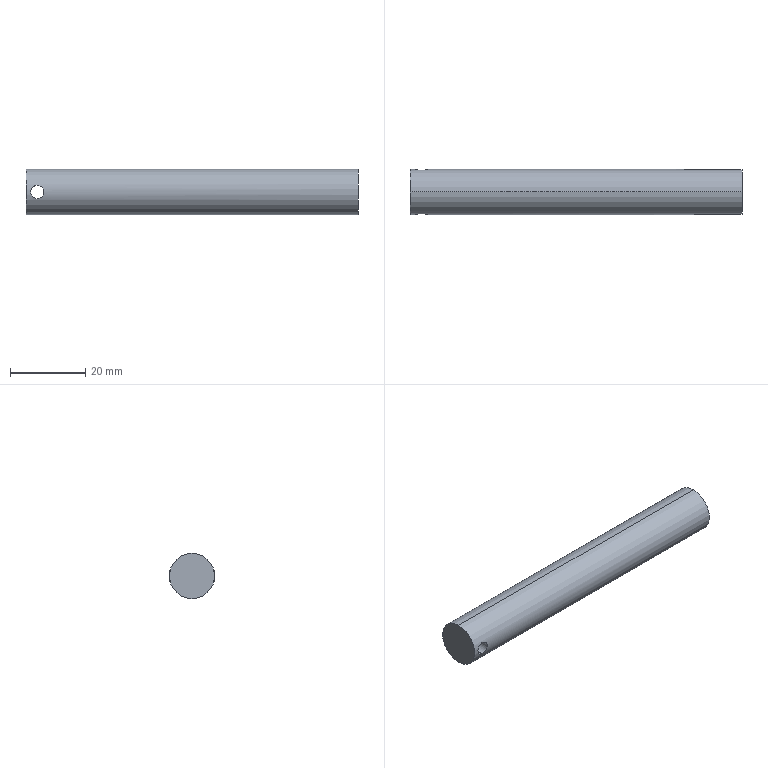Part | STEP file | Part 4 | 1 solid | 6 faces | box 88 x 12 x 12 mm | volume 9838 mm3 | cylinder 4 | plane 2 | commonest cylinder face diameters 3.5 x2 12 x2
STEP:
#1=CARTESIAN_POINT('',(0.,0.,0.));
#2=DIRECTION('',(0.,0.,1.));
#3=DIRECTION('',(1.,0.,0.));
#4=AXIS2_PLACEMENT_3D('',#1,#2,#3);
#5=CARTESIAN_POINT('',(3.,-5.739,1.75));
#6=VERTEX_POINT('',#5);
#7=CARTESIAN_POINT('',(3.,5.739,1.75));
#8=VERTEX_POINT('',#7);
#9=CARTESIAN_POINT('',(3.,-6.,1.75));
#10=DIRECTION('',(0.,1.,0.));
#11=VECTOR('',#10,1.);
#12=LINE('',#9,#11);
#13=CARTESIAN_POINT('',(3.,-6.,0.));
#14=DIRECTION('',(0.,1.,0.));
#15=DIRECTION('',(0.,0.,1.));
#16=AXIS2_PLACEMENT_3D('',#13,#14,#15);
#17=CYLINDRICAL_SURFACE('',#16,1.75);
#18=CARTESIAN_POINT('',(6.283,0.));
#19=DIRECTION('',(0.,1.));
#20=VECTOR('',#19,1.);
#21=LINE('',#18,#20);
#22=(GEOMETRIC_REPRESENTATION_CONTEXT(2)PARAMETRIC_REPRESENTATION_CONTEXT()REPRESENTATION_CONTEXT('',''));
#23=DEFINITIONAL_REPRESENTATION('',(#21),#22);
#24=PCURVE('',#17,#23);
#25=CARTESIAN_POINT('',(3.,-6.,0.));
#26=DIRECTION('',(0.,1.,0.));
#27=DIRECTION('',(0.,0.,1.));
#28=AXIS2_PLACEMENT_3D('',#25,#26,#27);
#29=CYLINDRICAL_SURFACE('',#28,1.75);
#30=CARTESIAN_POINT('',(0.,0.));
#31=DIRECTION('',(0.,1.));
#32=VECTOR('',#31,1.);
#33=LINE('',#30,#32);
#34=(GEOMETRIC_REPRESENTATION_CONTEXT(2)PARAMETRIC_REPRESENTATION_CONTEXT()REPRESENTATION_CONTEXT('',''));
#35=DEFINITIONAL_REPRESENTATION('',(#33),#34);
#36=PCURVE('',#29,#35);
#37=SURFACE_CURVE('',#12,(#24,#36),.PCURVE_S1.);
#38=EDGE_CURVE('',#6,#8,#37,.T.);
#39=ORIENTED_EDGE('',*,*,#38,.T.);
#40=CARTESIAN_POINT('',(3.,5.739,-1.75));
#41=VERTEX_POINT('',#40);
#42=CARTESIAN_POINT('',(3.,5.739,1.75));
#43=CARTESIAN_POINT('',(2.884,5.739,1.75));
#44=CARTESIAN_POINT('',(2.769,5.743,1.739));
#45=CARTESIAN_POINT('',(2.545,5.756,1.694));
#46=CARTESIAN_POINT('',(2.433,5.766,1.66));
#47=CARTESIAN_POINT('',(2.222,5.791,1.572));
#48=CARTESIAN_POINT('',(2.122,5.805,1.518));
#49=CARTESIAN_POINT('',(1.932,5.837,1.391));
#50=CARTESIAN_POINT('',(1.843,5.854,1.317));
#51=CARTESIAN_POINT('',(1.602,5.905,1.077));
#52=CARTESIAN_POINT('',(1.472,5.939,0.8824));
#53=CARTESIAN_POINT('',(1.34,5.974,0.5668));
#54=CARTESIAN_POINT('',(1.306,5.984,0.4558));
#55=CARTESIAN_POINT('',(1.261,5.997,0.2296));
#56=CARTESIAN_POINT('',(1.25,6.,0.1156));
#57=CARTESIAN_POINT('',(1.25,6.,-0.1141));
#58=CARTESIAN_POINT('',(1.261,5.997,-0.2308));
#59=CARTESIAN_POINT('',(1.307,5.984,-0.4558));
#60=CARTESIAN_POINT('',(1.34,5.974,-0.5652));
#61=CARTESIAN_POINT('',(1.472,5.938,-0.8843));
#62=CARTESIAN_POINT('',(1.601,5.905,-1.076));
#63=CARTESIAN_POINT('',(1.844,5.854,-1.319));
#64=CARTESIAN_POINT('',(1.932,5.837,-1.391));
#65=CARTESIAN_POINT('',(2.121,5.805,-1.517));
#66=CARTESIAN_POINT('',(2.223,5.79,-1.572));
#67=CARTESIAN_POINT('',(2.434,5.766,-1.66));
#68=CARTESIAN_POINT('',(2.543,5.756,-1.693));
#69=CARTESIAN_POINT('',(2.769,5.743,-1.739));
#70=CARTESIAN_POINT('',(2.885,5.739,-1.75));
#71=CARTESIAN_POINT('',(3.,5.739,-1.75));
#72=B_SPLINE_CURVE_WITH_KNOTS('',3,(#42,#43,#44,#45,#46,#47,#48,#49,#50,#51,#52,#53,#54,#55,#56,#57,#58,#59,#60,#61,#62,#63,#64,#65,#66,#67,#68,#69,#70,#71),.UNSPECIFIED.,.F.,.F.,(4,2,2,2,2,2,2,2,2,2,2,2,2,2,4),(0.,0.0003438,0.0006877,0.001031,0.001375,0.002063,0.002407,0.002751,0.003094,0.003438,0.004126,0.00447,0.004814,0.005157,0.005501),.UNSPECIFIED.);
#73=CARTESIAN_POINT('',(6.283,11.739));
#74=CARTESIAN_POINT('',(6.267,11.739));
#75=CARTESIAN_POINT('',(6.235,11.74));
#76=CARTESIAN_POINT('',(6.187,11.741));
#77=CARTESIAN_POINT('',(6.14,11.744));
#78=CARTESIAN_POINT('',(6.092,11.749));
#79=CARTESIAN_POINT('',(6.044,11.754));
#80=CARTESIAN_POINT('',(5.996,11.76));
#81=CARTESIAN_POINT('',(5.949,11.768));
#82=CARTESIAN_POINT('',(5.901,11.776));
#83=CARTESIAN_POINT('',(5.853,11.785));
#84=CARTESIAN_POINT('',(5.806,11.795));
#85=CARTESIAN_POINT('',(5.759,11.806));
#86=CARTESIAN_POINT('',(5.711,11.817));
#87=CARTESIAN_POINT('',(5.664,11.828));
#88=CARTESIAN_POINT('',(5.616,11.84));
#89=CARTESIAN_POINT('',(5.569,11.853));
#90=CARTESIAN_POINT('',(5.521,11.865));
#91=CARTESIAN_POINT('',(5.474,11.877));
#92=CARTESIAN_POINT('',(5.427,11.889));
#93=CARTESIAN_POINT('',(5.379,11.902));
#94=CARTESIAN_POINT('',(5.332,11.913));
#95=CARTESIAN_POINT('',(5.284,11.925));
#96=CARTESIAN_POINT('',(5.237,11.936));
#97=CARTESIAN_POINT('',(5.189,11.946));
#98=CARTESIAN_POINT('',(5.142,11.956));
#99=CARTESIAN_POINT('',(5.095,11.965));
#100=CARTESIAN_POINT('',(5.047,11.973));
#101=CARTESIAN_POINT('',(4.999,11.98));
#102=CARTESIAN_POINT('',(4.951,11.986));
#103=CARTESIAN_POINT('',(4.903,11.991));
#104=CARTESIAN_POINT('',(4.856,11.995));
#105=CARTESIAN_POINT('',(4.808,11.998));
#106=CARTESIAN_POINT('',(4.76,12.));
#107=CARTESIAN_POINT('',(4.713,12.));
#108=CARTESIAN_POINT('',(4.665,12.));
#109=CARTESIAN_POINT('',(4.617,11.998));
#110=CARTESIAN_POINT('',(4.569,11.995));
#111=CARTESIAN_POINT('',(4.521,11.991));
#112=CARTESIAN_POINT('',(4.473,11.986));
#113=CARTESIAN_POINT('',(4.426,11.98));
#114=CARTESIAN_POINT('',(4.378,11.973));
#115=CARTESIAN_POINT('',(4.331,11.965));
#116=CARTESIAN_POINT('',(4.283,11.956));
#117=CARTESIAN_POINT('',(4.235,11.946));
#118=CARTESIAN_POINT('',(4.187,11.936));
#119=CARTESIAN_POINT('',(4.14,11.925));
#120=CARTESIAN_POINT('',(4.093,11.913));
#121=CARTESIAN_POINT('',(4.045,11.901));
#122=CARTESIAN_POINT('',(3.998,11.889));
#123=CARTESIAN_POINT('',(3.95,11.877));
#124=CARTESIAN_POINT('',(3.903,11.865));
#125=CARTESIAN_POINT('',(3.856,11.852));
#126=CARTESIAN_POINT('',(3.808,11.84));
#127=CARTESIAN_POINT('',(3.761,11.828));
#128=CARTESIAN_POINT('',(3.714,11.817));
#129=CARTESIAN_POINT('',(3.666,11.806));
#130=CARTESIAN_POINT('',(3.619,11.795));
#131=CARTESIAN_POINT('',(3.571,11.785));
#132=CARTESIAN_POINT('',(3.523,11.776));
#133=CARTESIAN_POINT('',(3.476,11.768));
#134=CARTESIAN_POINT('',(3.429,11.76));
#135=CARTESIAN_POINT('',(3.381,11.754));
#136=CARTESIAN_POINT('',(3.333,11.749));
#137=CARTESIAN_POINT('',(3.285,11.744));
#138=CARTESIAN_POINT('',(3.237,11.741));
#139=CARTESIAN_POINT('',(3.189,11.74));
#140=CARTESIAN_POINT('',(3.157,11.739));
#141=CARTESIAN_POINT('',(3.142,11.739));
#142=B_SPLINE_CURVE_WITH_KNOTS('',3,(#73,#74,#75,#76,#77,#78,#79,#80,#81,#82,#83,#84,#85,#86,#87,#88,#89,#90,#91,#92,#93,#94,#95,#96,#97,#98,#99,#100,#101,#102,#103,#104,#105,#106,#107,#108,#109,#110,#111,#112,#113,#114,#115,#116,#117,#118,#119,#120,#121,#122,#123,#124,#125,#126,#127,#128,#129,#130,#131,#132,#133,#134,#135,#136,#137,#138,#139,#140,#141),.UNSPECIFIED.,.F.,.F.,(4,1,1,1,1,1,1,1,1,1,1,1,1,1,1,1,1,1,1,1,1,1,1,1,1,1,1,1,1,1,1,1,1,1,1,1,1,1,1,1,1,1,1,1,1,1,1,1,1,1,1,1,1,1,1,1,1,1,1,1,1,1,1,1,1,1,4),(0.,0.00008335,0.0001667,0.0002501,0.0003334,0.0004168,0.0005001,0.0005835,0.0006668,0.0007502,0.0008335,0.0009169,0.001,0.001084,0.001167,0.00125,0.001334,0.001417,0.0015,0.001584,0.001667,0.00175,0.001834,0.001917,0.002,0.002084,0.002167,0.002251,0.002334,0.002417,0.002501,0.002584,0.002667,0.002751,0.002834,0.002917,0.003001,0.003084,0.003167,0.003251,0.003334,0.003417,0.003501,0.003584,0.003668,0.003751,0.003834,0.003918,0.004001,0.004084,0.004168,0.004251,0.004334,0.004418,0.004501,0.004584,0.004668,0.004751,0.004834,0.004918,0.005001,0.005085,0.005168,0.005251,0.005335,0.005418,0.005501),.QUASI_UNIFORM_KNOTS.);
#143=(GEOMETRIC_REPRESENTATION_CONTEXT(2)PARAMETRIC_REPRESENTATION_CONTEXT()REPRESENTATION_CONTEXT('',''));
#144=DEFINITIONAL_REPRESENTATION('',(#142),#143);
#145=PCURVE('',#17,#144);
#146=CARTESIAN_POINT('',(-269.087,0.,0.));
#147=DIRECTION('',(-1.,0.,0.));
#148=DIRECTION('',(0.,0.,1.));
#149=AXIS2_PLACEMENT_3D('',#146,#147,#148);
#150=CYLINDRICAL_SURFACE('',#149,6.);
#151=CARTESIAN_POINT('',(1.275,-272.087));
#152=CARTESIAN_POINT('',(1.275,-272.058));
#153=CARTESIAN_POINT('',(1.275,-272.002));
#154=CARTESIAN_POINT('',(1.276,-271.919));
#155=CARTESIAN_POINT('',(1.278,-271.836));
#156=CARTESIAN_POINT('',(1.28,-271.754));
#157=CARTESIAN_POINT('',(1.283,-271.672));
#158=CARTESIAN_POINT('',(1.287,-271.591));
#159=CARTESIAN_POINT('',(1.292,-271.512));
#160=CARTESIAN_POINT('',(1.297,-271.433));
#161=CARTESIAN_POINT('',(1.302,-271.357));
#162=CARTESIAN_POINT('',(1.309,-271.282));
#163=CARTESIAN_POINT('',(1.316,-271.21));
#164=CARTESIAN_POINT('',(1.323,-271.139));
#165=CARTESIAN_POINT('',(1.331,-271.07));
#166=CARTESIAN_POINT('',(1.34,-271.004));
#167=CARTESIAN_POINT('',(1.349,-270.939));
#168=CARTESIAN_POINT('',(1.358,-270.878));
#169=CARTESIAN_POINT('',(1.368,-270.82));
#170=CARTESIAN_POINT('',(1.378,-270.764));
#171=CARTESIAN_POINT('',(1.389,-270.711));
#172=CARTESIAN_POINT('',(1.401,-270.661));
#173=CARTESIAN_POINT('',(1.412,-270.615));
#174=CARTESIAN_POINT('',(1.424,-270.571));
#175=CARTESIAN_POINT('',(1.436,-270.532));
#176=CARTESIAN_POINT('',(1.449,-270.495));
#177=CARTESIAN_POINT('',(1.462,-270.462));
#178=CARTESIAN_POINT('',(1.475,-270.433));
#179=CARTESIAN_POINT('',(1.488,-270.408));
#180=CARTESIAN_POINT('',(1.502,-270.386));
#181=CARTESIAN_POINT('',(1.515,-270.368));
#182=CARTESIAN_POINT('',(1.529,-270.354));
#183=CARTESIAN_POINT('',(1.543,-270.344));
#184=CARTESIAN_POINT('',(1.557,-270.338));
#185=CARTESIAN_POINT('',(1.571,-270.336));
#186=CARTESIAN_POINT('',(1.585,-270.338));
#187=CARTESIAN_POINT('',(1.599,-270.344));
#188=CARTESIAN_POINT('',(1.613,-270.354));
#189=CARTESIAN_POINT('',(1.626,-270.368));
#190=CARTESIAN_POINT('',(1.64,-270.386));
#191=CARTESIAN_POINT('',(1.653,-270.407));
#192=CARTESIAN_POINT('',(1.667,-270.433));
#193=CARTESIAN_POINT('',(1.68,-270.462));
#194=CARTESIAN_POINT('',(1.693,-270.495));
#195=CARTESIAN_POINT('',(1.705,-270.532));
#196=CARTESIAN_POINT('',(1.718,-270.572));
#197=CARTESIAN_POINT('',(1.73,-270.615));
#198=CARTESIAN_POINT('',(1.741,-270.662));
#199=CARTESIAN_POINT('',(1.752,-270.711));
#200=CARTESIAN_POINT('',(1.763,-270.764));
#201=CARTESIAN_POINT('',(1.774,-270.82));
#202=CARTESIAN_POINT('',(1.784,-270.879));
#203=CARTESIAN_POINT('',(1.793,-270.94));
#204=CARTESIAN_POINT('',(1.802,-271.004));
#205=CARTESIAN_POINT('',(1.811,-271.07));
#206=CARTESIAN_POINT('',(1.819,-271.138));
#207=CARTESIAN_POINT('',(1.826,-271.209));
#208=CARTESIAN_POINT('',(1.833,-271.283));
#209=CARTESIAN_POINT('',(1.839,-271.358));
#210=CARTESIAN_POINT('',(1.845,-271.434));
#211=CARTESIAN_POINT('',(1.85,-271.512));
#212=CARTESIAN_POINT('',(1.854,-271.591));
#213=CARTESIAN_POINT('',(1.858,-271.671));
#214=CARTESIAN_POINT('',(1.861,-271.753));
#215=CARTESIAN_POINT('',(1.864,-271.836));
#216=CARTESIAN_POINT('',(1.865,-271.919));
#217=CARTESIAN_POINT('',(1.867,-272.003));
#218=CARTESIAN_POINT('',(1.867,-272.059));
#219=CARTESIAN_POINT('',(1.867,-272.087));
#220=B_SPLINE_CURVE_WITH_KNOTS('',3,(#151,#152,#153,#154,#155,#156,#157,#158,#159,#160,#161,#162,#163,#164,#165,#166,#167,#168,#169,#170,#171,#172,#173,#174,#175,#176,#177,#178,#179,#180,#181,#182,#183,#184,#185,#186,#187,#188,#189,#190,#191,#192,#193,#194,#195,#196,#197,#198,#199,#200,#201,#202,#203,#204,#205,#206,#207,#208,#209,#210,#211,#212,#213,#214,#215,#216,#217,#218,#219),.UNSPECIFIED.,.F.,.F.,(4,1,1,1,1,1,1,1,1,1,1,1,1,1,1,1,1,1,1,1,1,1,1,1,1,1,1,1,1,1,1,1,1,1,1,1,1,1,1,1,1,1,1,1,1,1,1,1,1,1,1,1,1,1,1,1,1,1,1,1,1,1,1,1,1,1,4),(0.,0.00008335,0.0001667,0.0002501,0.0003334,0.0004168,0.0005001,0.0005835,0.0006668,0.0007502,0.0008335,0.0009169,0.001,0.001084,0.001167,0.00125,0.001334,0.001417,0.0015,0.001584,0.001667,0.00175,0.001834,0.001917,0.002,0.002084,0.002167,0.002251,0.002334,0.002417,0.002501,0.002584,0.002667,0.002751,0.002834,0.002917,0.003001,0.003084,0.003167,0.003251,0.003334,0.003417,0.003501,0.003584,0.003668,0.003751,0.003834,0.003918,0.004001,0.004084,0.004168,0.004251,0.004334,0.004418,0.004501,0.004584,0.004668,0.004751,0.004834,0.004918,0.005001,0.005085,0.005168,0.005251,0.005335,0.005418,0.005501),.QUASI_UNIFORM_KNOTS.);
#221=(GEOMETRIC_REPRESENTATION_CONTEXT(2)PARAMETRIC_REPRESENTATION_CONTEXT()REPRESENTATION_CONTEXT('',''));
#222=DEFINITIONAL_REPRESENTATION('',(#220),#221);
#223=PCURVE('',#150,#222);
#224=SURFACE_CURVE('',#72,(#145,#223),.PCURVE_S1.);
#225=EDGE_CURVE('',#8,#41,#224,.T.);
#226=ORIENTED_EDGE('',*,*,#225,.T.);
#227=CARTESIAN_POINT('',(3.,-5.739,-1.75));
#228=VERTEX_POINT('',#227);
#229=CARTESIAN_POINT('',(3.,-6.,-1.75));
#230=DIRECTION('',(0.,1.,0.));
#231=VECTOR('',#230,1.);
#232=LINE('',#229,#231);
#233=CARTESIAN_POINT('',(3.142,0.));
#234=DIRECTION('',(0.,1.));
#235=VECTOR('',#234,1.);
#236=LINE('',#233,#235);
#237=(GEOMETRIC_REPRESENTATION_CONTEXT(2)PARAMETRIC_REPRESENTATION_CONTEXT()REPRESENTATION_CONTEXT('',''));
#238=DEFINITIONAL_REPRESENTATION('',(#236),#237);
#239=PCURVE('',#17,#238);
#240=CARTESIAN_POINT('',(3.142,0.));
#241=DIRECTION('',(0.,1.));
#242=VECTOR('',#241,1.);
#243=LINE('',#240,#242);
#244=(GEOMETRIC_REPRESENTATION_CONTEXT(2)PARAMETRIC_REPRESENTATION_CONTEXT()REPRESENTATION_CONTEXT('',''));
#245=DEFINITIONAL_REPRESENTATION('',(#243),#244);
#246=PCURVE('',#29,#245);
#247=SURFACE_CURVE('',#232,(#239,#246),.PCURVE_S1.);
#248=EDGE_CURVE('',#228,#41,#247,.T.);
#249=ORIENTED_EDGE('',*,*,#248,.F.);
#250=CARTESIAN_POINT('',(3.,-5.739,-1.75));
#251=CARTESIAN_POINT('',(2.885,-5.739,-1.75));
#252=CARTESIAN_POINT('',(2.771,-5.743,-1.739));
#253=CARTESIAN_POINT('',(2.545,-5.756,-1.694));
#254=CARTESIAN_POINT('',(2.434,-5.766,-1.66));
#255=CARTESIAN_POINT('',(2.117,-5.803,-1.528));
#256=CARTESIAN_POINT('',(1.923,-5.837,-1.398));
#257=CARTESIAN_POINT('',(1.682,-5.888,-1.157));
#258=CARTESIAN_POINT('',(1.609,-5.905,-1.068));
#259=CARTESIAN_POINT('',(1.482,-5.936,-0.8782));
#260=CARTESIAN_POINT('',(1.428,-5.95,-0.778));
#261=CARTESIAN_POINT('',(1.34,-5.974,-0.5669));
#262=CARTESIAN_POINT('',(1.306,-5.984,-0.4551));
#263=CARTESIAN_POINT('',(1.261,-5.997,-0.2299));
#264=CARTESIAN_POINT('',(1.25,-6.,-0.1154));
#265=CARTESIAN_POINT('',(1.25,-6.,0.1172));
#266=CARTESIAN_POINT('',(1.262,-5.997,0.2314));
#267=CARTESIAN_POINT('',(1.307,-5.984,0.4559));
#268=CARTESIAN_POINT('',(1.341,-5.974,0.5674));
#269=CARTESIAN_POINT('',(1.429,-5.95,0.779));
#270=CARTESIAN_POINT('',(1.483,-5.936,0.8793));
#271=CARTESIAN_POINT('',(1.61,-5.905,1.069));
#272=CARTESIAN_POINT('',(1.683,-5.888,1.158));
#273=CARTESIAN_POINT('',(1.924,-5.837,1.399));
#274=CARTESIAN_POINT('',(2.118,-5.803,1.529));
#275=CARTESIAN_POINT('',(2.434,-5.766,1.66));
#276=CARTESIAN_POINT('',(2.545,-5.756,1.694));
#277=CARTESIAN_POINT('',(2.771,-5.743,1.739));
#278=CARTESIAN_POINT('',(2.885,-5.739,1.75));
#279=CARTESIAN_POINT('',(3.,-5.739,1.75));
#280=B_SPLINE_CURVE_WITH_KNOTS('',3,(#250,#251,#252,#253,#254,#255,#256,#257,#258,#259,#260,#261,#262,#263,#264,#265,#266,#267,#268,#269,#270,#271,#272,#273,#274,#275,#276,#277,#278,#279),.UNSPECIFIED.,.F.,.F.,(4,2,2,2,2,2,2,2,2,2,2,2,2,2,4),(0.008251,0.008595,0.008939,0.009627,0.009971,0.01031,0.01066,0.011,0.01135,0.01169,0.01203,0.01238,0.01307,0.01341,0.01375),.UNSPECIFIED.);
#281=CARTESIAN_POINT('',(3.142,0.2609));
#282=CARTESIAN_POINT('',(3.158,0.2609));
#283=CARTESIAN_POINT('',(3.189,0.2605));
#284=CARTESIAN_POINT('',(3.237,0.2587));
#285=CARTESIAN_POINT('',(3.285,0.2556));
#286=CARTESIAN_POINT('',(3.332,0.2515));
#287=CARTESIAN_POINT('',(3.38,0.2462));
#288=CARTESIAN_POINT('',(3.428,0.2398));
#289=CARTESIAN_POINT('',(3.476,0.2323));
#290=CARTESIAN_POINT('',(3.524,0.224));
#291=CARTESIAN_POINT('',(3.571,0.2149));
#292=CARTESIAN_POINT('',(3.619,0.205));
#293=CARTESIAN_POINT('',(3.666,0.1944));
#294=CARTESIAN_POINT('',(3.714,0.1832));
#295=CARTESIAN_POINT('',(3.761,0.1716));
#296=CARTESIAN_POINT('',(3.809,0.1597));
#297=CARTESIAN_POINT('',(3.856,0.1475));
#298=CARTESIAN_POINT('',(3.903,0.1352));
#299=CARTESIAN_POINT('',(3.95,0.1229));
#300=CARTESIAN_POINT('',(3.998,0.1106));
#301=CARTESIAN_POINT('',(4.045,0.09843));
#302=CARTESIAN_POINT('',(4.093,0.08657));
#303=CARTESIAN_POINT('',(4.141,0.07514));
#304=CARTESIAN_POINT('',(4.188,0.06425));
#305=CARTESIAN_POINT('',(4.235,0.05398));
#306=CARTESIAN_POINT('',(4.282,0.04439));
#307=CARTESIAN_POINT('',(4.33,0.03553));
#308=CARTESIAN_POINT('',(4.378,0.02747));
#309=CARTESIAN_POINT('',(4.426,0.02031));
#310=CARTESIAN_POINT('',(4.474,0.01413));
#311=CARTESIAN_POINT('',(4.521,0.009023));
#312=CARTESIAN_POINT('',(4.569,0.005024));
#313=CARTESIAN_POINT('',(4.617,0.002134));
#314=CARTESIAN_POINT('',(4.665,0.0003848));
#315=CARTESIAN_POINT('',(4.713,-0.0001984));
#316=CARTESIAN_POINT('',(4.761,0.0004093));
#317=CARTESIAN_POINT('',(4.809,0.002179));
#318=CARTESIAN_POINT('',(4.857,0.005084));
#319=CARTESIAN_POINT('',(4.904,0.00909));
#320=CARTESIAN_POINT('',(4.952,0.01419));
#321=CARTESIAN_POINT('',(5.,0.02037));
#322=CARTESIAN_POINT('',(5.048,0.02754));
#323=CARTESIAN_POINT('',(5.095,0.03561));
#324=CARTESIAN_POINT('',(5.143,0.0445));
#325=CARTESIAN_POINT('',(5.19,0.05412));
#326=CARTESIAN_POINT('',(5.238,0.06441));
#327=CARTESIAN_POINT('',(5.285,0.0753));
#328=CARTESIAN_POINT('',(5.332,0.08673));
#329=CARTESIAN_POINT('',(5.38,0.09859));
#330=CARTESIAN_POINT('',(5.428,0.1107));
#331=CARTESIAN_POINT('',(5.475,0.1231));
#332=CARTESIAN_POINT('',(5.522,0.1354));
#333=CARTESIAN_POINT('',(5.569,0.1477));
#334=CARTESIAN_POINT('',(5.617,0.1598));
#335=CARTESIAN_POINT('',(5.664,0.1718));
#336=CARTESIAN_POINT('',(5.712,0.1834));
#337=CARTESIAN_POINT('',(5.759,0.1945));
#338=CARTESIAN_POINT('',(5.807,0.2051));
#339=CARTESIAN_POINT('',(5.854,0.215));
#340=CARTESIAN_POINT('',(5.901,0.2241));
#341=CARTESIAN_POINT('',(5.949,0.2324));
#342=CARTESIAN_POINT('',(5.997,0.2398));
#343=CARTESIAN_POINT('',(6.045,0.2462));
#344=CARTESIAN_POINT('',(6.093,0.2515));
#345=CARTESIAN_POINT('',(6.14,0.2557));
#346=CARTESIAN_POINT('',(6.188,0.2587));
#347=CARTESIAN_POINT('',(6.236,0.2605));
#348=CARTESIAN_POINT('',(6.267,0.2609));
#349=CARTESIAN_POINT('',(6.283,0.2609));
#350=B_SPLINE_CURVE_WITH_KNOTS('',3,(#281,#282,#283,#284,#285,#286,#287,#288,#289,#290,#291,#292,#293,#294,#295,#296,#297,#298,#299,#300,#301,#302,#303,#304,#305,#306,#307,#308,#309,#310,#311,#312,#313,#314,#315,#316,#317,#318,#319,#320,#321,#322,#323,#324,#325,#326,#327,#328,#329,#330,#331,#332,#333,#334,#335,#336,#337,#338,#339,#340,#341,#342,#343,#344,#345,#346,#347,#348,#349),.UNSPECIFIED.,.F.,.F.,(4,1,1,1,1,1,1,1,1,1,1,1,1,1,1,1,1,1,1,1,1,1,1,1,1,1,1,1,1,1,1,1,1,1,1,1,1,1,1,1,1,1,1,1,1,1,1,1,1,1,1,1,1,1,1,1,1,1,1,1,1,1,1,1,1,1,4),(0.008251,0.008335,0.008418,0.008502,0.008585,0.008668,0.008752,0.008835,0.008918,0.009002,0.009085,0.009168,0.009252,0.009335,0.009418,0.009502,0.009585,0.009668,0.009752,0.009835,0.009919,0.01,0.01009,0.01017,0.01025,0.01034,0.01042,0.0105,0.01059,0.01067,0.01075,0.01084,0.01092,0.011,0.01109,0.01117,0.01125,0.01134,0.01142,0.0115,0.01159,0.01167,0.01175,0.01184,0.01192,0.012,0.01209,0.01217,0.01225,0.01234,0.01242,0.0125,0.01259,0.01267,0.01275,0.01284,0.01292,0.013,0.01309,0.01317,0.01325,0.01334,0.01342,0.0135,0.01359,0.01367,0.01375),.QUASI_UNIFORM_KNOTS.);
#351=(GEOMETRIC_REPRESENTATION_CONTEXT(2)PARAMETRIC_REPRESENTATION_CONTEXT()REPRESENTATION_CONTEXT('',''));
#352=DEFINITIONAL_REPRESENTATION('',(#350),#351);
#353=PCURVE('',#17,#352);
#354=CARTESIAN_POINT('',(-269.087,0.,0.));
#355=DIRECTION('',(-1.,0.,0.));
#356=DIRECTION('',(0.,0.,1.));
#357=AXIS2_PLACEMENT_3D('',#354,#355,#356);
#358=CYLINDRICAL_SURFACE('',#357,6.);
#359=CARTESIAN_POINT('',(4.416,-272.087));
#360=CARTESIAN_POINT('',(4.416,-272.059));
#361=CARTESIAN_POINT('',(4.417,-272.003));
#362=CARTESIAN_POINT('',(4.418,-271.92));
#363=CARTESIAN_POINT('',(4.419,-271.837));
#364=CARTESIAN_POINT('',(4.422,-271.755));
#365=CARTESIAN_POINT('',(4.425,-271.673));
#366=CARTESIAN_POINT('',(4.429,-271.592));
#367=CARTESIAN_POINT('',(4.433,-271.512));
#368=CARTESIAN_POINT('',(4.438,-271.434));
#369=CARTESIAN_POINT('',(4.444,-271.357));
#370=CARTESIAN_POINT('',(4.45,-271.283));
#371=CARTESIAN_POINT('',(4.457,-271.21));
#372=CARTESIAN_POINT('',(4.465,-271.139));
#373=CARTESIAN_POINT('',(4.473,-271.07));
#374=CARTESIAN_POINT('',(4.481,-271.004));
#375=CARTESIAN_POINT('',(4.49,-270.94));
#376=CARTESIAN_POINT('',(4.5,-270.878));
#377=CARTESIAN_POINT('',(4.51,-270.82));
#378=CARTESIAN_POINT('',(4.52,-270.764));
#379=CARTESIAN_POINT('',(4.531,-270.711));
#380=CARTESIAN_POINT('',(4.542,-270.661));
#381=CARTESIAN_POINT('',(4.554,-270.614));
#382=CARTESIAN_POINT('',(4.566,-270.571));
#383=CARTESIAN_POINT('',(4.578,-270.532));
#384=CARTESIAN_POINT('',(4.59,-270.495));
#385=CARTESIAN_POINT('',(4.603,-270.462));
#386=CARTESIAN_POINT('',(4.616,-270.433));
#387=CARTESIAN_POINT('',(4.63,-270.407));
#388=CARTESIAN_POINT('',(4.643,-270.386));
#389=CARTESIAN_POINT('',(4.657,-270.368));
#390=CARTESIAN_POINT('',(4.671,-270.354));
#391=CARTESIAN_POINT('',(4.685,-270.344));
#392=CARTESIAN_POINT('',(4.698,-270.338));
#393=CARTESIAN_POINT('',(4.713,-270.336));
#394=CARTESIAN_POINT('',(4.727,-270.338));
#395=CARTESIAN_POINT('',(4.741,-270.344));
#396=CARTESIAN_POINT('',(4.754,-270.354));
#397=CARTESIAN_POINT('',(4.768,-270.368));
#398=CARTESIAN_POINT('',(4.782,-270.386));
#399=CARTESIAN_POINT('',(4.795,-270.408));
#400=CARTESIAN_POINT('',(4.809,-270.433));
#401=CARTESIAN_POINT('',(4.822,-270.463));
#402=CARTESIAN_POINT('',(4.834,-270.496));
#403=CARTESIAN_POINT('',(4.847,-270.532));
#404=CARTESIAN_POINT('',(4.859,-270.572));
#405=CARTESIAN_POINT('',(4.871,-270.615));
#406=CARTESIAN_POINT('',(4.883,-270.662));
#407=CARTESIAN_POINT('',(4.894,-270.712));
#408=CARTESIAN_POINT('',(4.905,-270.765));
#409=CARTESIAN_POINT('',(4.915,-270.821));
#410=CARTESIAN_POINT('',(4.925,-270.879));
#411=CARTESIAN_POINT('',(4.935,-270.941));
#412=CARTESIAN_POINT('',(4.944,-271.005));
#413=CARTESIAN_POINT('',(4.952,-271.071));
#414=CARTESIAN_POINT('',(4.96,-271.14));
#415=CARTESIAN_POINT('',(4.968,-271.211));
#416=CARTESIAN_POINT('',(4.975,-271.284));
#417=CARTESIAN_POINT('',(4.981,-271.358));
#418=CARTESIAN_POINT('',(4.987,-271.434));
#419=CARTESIAN_POINT('',(4.992,-271.512));
#420=CARTESIAN_POINT('',(4.996,-271.592));
#421=CARTESIAN_POINT('',(5.,-271.673));
#422=CARTESIAN_POINT('',(5.003,-271.755));
#423=CARTESIAN_POINT('',(5.005,-271.837));
#424=CARTESIAN_POINT('',(5.007,-271.92));
#425=CARTESIAN_POINT('',(5.008,-272.003));
#426=CARTESIAN_POINT('',(5.008,-272.059));
#427=CARTESIAN_POINT('',(5.008,-272.087));
#428=B_SPLINE_CURVE_WITH_KNOTS('',3,(#359,#360,#361,#362,#363,#364,#365,#366,#367,#368,#369,#370,#371,#372,#373,#374,#375,#376,#377,#378,#379,#380,#381,#382,#383,#384,#385,#386,#387,#388,#389,#390,#391,#392,#393,#394,#395,#396,#397,#398,#399,#400,#401,#402,#403,#404,#405,#406,#407,#408,#409,#410,#411,#412,#413,#414,#415,#416,#417,#418,#419,#420,#421,#422,#423,#424,#425,#426,#427),.UNSPECIFIED.,.F.,.F.,(4,1,1,1,1,1,1,1,1,1,1,1,1,1,1,1,1,1,1,1,1,1,1,1,1,1,1,1,1,1,1,1,1,1,1,1,1,1,1,1,1,1,1,1,1,1,1,1,1,1,1,1,1,1,1,1,1,1,1,1,1,1,1,1,1,1,4),(0.008251,0.008335,0.008418,0.008502,0.008585,0.008668,0.008752,0.008835,0.008918,0.009002,0.009085,0.009168,0.009252,0.009335,0.009418,0.009502,0.009585,0.009668,0.009752,0.009835,0.009919,0.01,0.01009,0.01017,0.01025,0.01034,0.01042,0.0105,0.01059,0.01067,0.01075,0.01084,0.01092,0.011,0.01109,0.01117,0.01125,0.01134,0.01142,0.0115,0.01159,0.01167,0.01175,0.01184,0.01192,0.012,0.01209,0.01217,0.01225,0.01234,0.01242,0.0125,0.01259,0.01267,0.01275,0.01284,0.01292,0.013,0.01309,0.01317,0.01325,0.01334,0.01342,0.0135,0.01359,0.01367,0.01375),.QUASI_UNIFORM_KNOTS.);
#429=(GEOMETRIC_REPRESENTATION_CONTEXT(2)PARAMETRIC_REPRESENTATION_CONTEXT()REPRESENTATION_CONTEXT('',''));
#430=DEFINITIONAL_REPRESENTATION('',(#428),#429);
#431=PCURVE('',#358,#430);
#432=SURFACE_CURVE('',#280,(#353,#431),.PCURVE_S1.);
#433=EDGE_CURVE('',#228,#6,#432,.T.);
#434=ORIENTED_EDGE('',*,*,#433,.T.);
#435=EDGE_LOOP('',(#39,#226,#249,#434));
#436=FACE_BOUND('',#435,.F.);
#437=ADVANCED_FACE('',(#436),#17,.F.);
#438=ORIENTED_EDGE('',*,*,#225,.T.);
#439=CARTESIAN_POINT('',(3.,5.739,-1.75));
#440=CARTESIAN_POINT('',(3.229,5.739,-1.75));
#441=CARTESIAN_POINT('',(3.461,5.754,-1.704));
#442=CARTESIAN_POINT('',(3.777,5.791,-1.572));
#443=CARTESIAN_POINT('',(3.879,5.805,-1.517));
#444=CARTESIAN_POINT('',(4.069,5.837,-1.391));
#445=CARTESIAN_POINT('',(4.156,5.854,-1.319));
#446=CARTESIAN_POINT('',(4.318,5.888,-1.157));
#447=CARTESIAN_POINT('',(4.391,5.905,-1.068));
#448=CARTESIAN_POINT('',(4.517,5.936,-0.8793));
#449=CARTESIAN_POINT('',(4.571,5.95,-0.7789));
#450=CARTESIAN_POINT('',(4.66,5.974,-0.5654));
#451=CARTESIAN_POINT('',(4.693,5.984,-0.456));
#452=CARTESIAN_POINT('',(4.738,5.997,-0.2317));
#453=CARTESIAN_POINT('',(4.75,6.,-0.1155));
#454=CARTESIAN_POINT('',(4.75,6.,0.1152));
#455=CARTESIAN_POINT('',(4.739,5.997,0.2292));
#456=CARTESIAN_POINT('',(4.694,5.984,0.4546));
#457=CARTESIAN_POINT('',(4.66,5.974,0.5662));
#458=CARTESIAN_POINT('',(4.528,5.939,0.8825));
#459=CARTESIAN_POINT('',(4.398,5.905,1.077));
#460=CARTESIAN_POINT('',(4.158,5.854,1.317));
#461=CARTESIAN_POINT('',(4.068,5.837,1.391));
#462=CARTESIAN_POINT('',(3.879,5.805,1.518));
#463=CARTESIAN_POINT('',(3.778,5.791,1.571));
#464=CARTESIAN_POINT('',(3.568,5.766,1.659));
#465=CARTESIAN_POINT('',(3.456,5.756,1.693));
#466=CARTESIAN_POINT('',(3.231,5.743,1.739));
#467=CARTESIAN_POINT('',(3.116,5.739,1.75));
#468=CARTESIAN_POINT('',(3.,5.739,1.75));
#469=B_SPLINE_CURVE_WITH_KNOTS('',3,(#439,#440,#441,#442,#443,#444,#445,#446,#447,#448,#449,#450,#451,#452,#453,#454,#455,#456,#457,#458,#459,#460,#461,#462,#463,#464,#465,#466,#467,#468),.UNSPECIFIED.,.F.,.F.,(4,2,2,2,2,2,2,2,2,2,2,2,2,2,4),(0.005501,0.006189,0.006532,0.006876,0.00722,0.007564,0.007907,0.008251,0.008595,0.008939,0.009626,0.00997,0.01031,0.01066,0.011),.UNSPECIFIED.);
#470=CARTESIAN_POINT('',(1.867,-272.087));
#471=CARTESIAN_POINT('',(1.867,-272.114));
#472=CARTESIAN_POINT('',(1.867,-272.17));
#473=CARTESIAN_POINT('',(1.865,-272.253));
#474=CARTESIAN_POINT('',(1.864,-272.336));
#475=CARTESIAN_POINT('',(1.861,-272.419));
#476=CARTESIAN_POINT('',(1.858,-272.501));
#477=CARTESIAN_POINT('',(1.854,-272.582));
#478=CARTESIAN_POINT('',(1.85,-272.661));
#479=CARTESIAN_POINT('',(1.845,-272.739));
#480=CARTESIAN_POINT('',(1.839,-272.815));
#481=CARTESIAN_POINT('',(1.833,-272.89));
#482=CARTESIAN_POINT('',(1.826,-272.964));
#483=CARTESIAN_POINT('',(1.819,-273.035));
#484=CARTESIAN_POINT('',(1.811,-273.103));
#485=CARTESIAN_POINT('',(1.802,-273.17));
#486=CARTESIAN_POINT('',(1.793,-273.233));
#487=CARTESIAN_POINT('',(1.784,-273.294));
#488=CARTESIAN_POINT('',(1.774,-273.353));
#489=CARTESIAN_POINT('',(1.763,-273.409));
#490=CARTESIAN_POINT('',(1.752,-273.462));
#491=CARTESIAN_POINT('',(1.741,-273.512));
#492=CARTESIAN_POINT('',(1.729,-273.558));
#493=CARTESIAN_POINT('',(1.718,-273.601));
#494=CARTESIAN_POINT('',(1.705,-273.641));
#495=CARTESIAN_POINT('',(1.693,-273.678));
#496=CARTESIAN_POINT('',(1.68,-273.711));
#497=CARTESIAN_POINT('',(1.667,-273.74));
#498=CARTESIAN_POINT('',(1.653,-273.766));
#499=CARTESIAN_POINT('',(1.64,-273.787));
#500=CARTESIAN_POINT('',(1.626,-273.805));
#501=CARTESIAN_POINT('',(1.613,-273.819));
#502=CARTESIAN_POINT('',(1.599,-273.829));
#503=CARTESIAN_POINT('',(1.585,-273.835));
#504=CARTESIAN_POINT('',(1.571,-273.837));
#505=CARTESIAN_POINT('',(1.557,-273.835));
#506=CARTESIAN_POINT('',(1.543,-273.829));
#507=CARTESIAN_POINT('',(1.529,-273.819));
#508=CARTESIAN_POINT('',(1.515,-273.806));
#509=CARTESIAN_POINT('',(1.502,-273.788));
#510=CARTESIAN_POINT('',(1.488,-273.766));
#511=CARTESIAN_POINT('',(1.475,-273.74));
#512=CARTESIAN_POINT('',(1.462,-273.711));
#513=CARTESIAN_POINT('',(1.449,-273.678));
#514=CARTESIAN_POINT('',(1.436,-273.642));
#515=CARTESIAN_POINT('',(1.424,-273.602));
#516=CARTESIAN_POINT('',(1.412,-273.558));
#517=CARTESIAN_POINT('',(1.401,-273.512));
#518=CARTESIAN_POINT('',(1.389,-273.462));
#519=CARTESIAN_POINT('',(1.378,-273.409));
#520=CARTESIAN_POINT('',(1.368,-273.354));
#521=CARTESIAN_POINT('',(1.358,-273.295));
#522=CARTESIAN_POINT('',(1.349,-273.234));
#523=CARTESIAN_POINT('',(1.34,-273.17));
#524=CARTESIAN_POINT('',(1.331,-273.103));
#525=CARTESIAN_POINT('',(1.323,-273.034));
#526=CARTESIAN_POINT('',(1.316,-272.964));
#527=CARTESIAN_POINT('',(1.309,-272.891));
#528=CARTESIAN_POINT('',(1.302,-272.817));
#529=CARTESIAN_POINT('',(1.297,-272.741));
#530=CARTESIAN_POINT('',(1.292,-272.662));
#531=CARTESIAN_POINT('',(1.287,-272.583));
#532=CARTESIAN_POINT('',(1.283,-272.501));
#533=CARTESIAN_POINT('',(1.28,-272.42));
#534=CARTESIAN_POINT('',(1.278,-272.337));
#535=CARTESIAN_POINT('',(1.276,-272.255));
#536=CARTESIAN_POINT('',(1.275,-272.171));
#537=CARTESIAN_POINT('',(1.275,-272.115));
#538=CARTESIAN_POINT('',(1.275,-272.087));
#539=B_SPLINE_CURVE_WITH_KNOTS('',3,(#470,#471,#472,#473,#474,#475,#476,#477,#478,#479,#480,#481,#482,#483,#484,#485,#486,#487,#488,#489,#490,#491,#492,#493,#494,#495,#496,#497,#498,#499,#500,#501,#502,#503,#504,#505,#506,#507,#508,#509,#510,#511,#512,#513,#514,#515,#516,#517,#518,#519,#520,#521,#522,#523,#524,#525,#526,#527,#528,#529,#530,#531,#532,#533,#534,#535,#536,#537,#538),.UNSPECIFIED.,.F.,.F.,(4,1,1,1,1,1,1,1,1,1,1,1,1,1,1,1,1,1,1,1,1,1,1,1,1,1,1,1,1,1,1,1,1,1,1,1,1,1,1,1,1,1,1,1,1,1,1,1,1,1,1,1,1,1,1,1,1,1,1,1,1,1,1,1,1,1,4),(0.005501,0.005585,0.005668,0.005751,0.005835,0.005918,0.006001,0.006085,0.006168,0.006251,0.006335,0.006418,0.006501,0.006585,0.006668,0.006751,0.006835,0.006918,0.007001,0.007085,0.007168,0.007251,0.007335,0.007418,0.007501,0.007585,0.007668,0.007751,0.007835,0.007918,0.008001,0.008084,0.008168,0.008251,0.008334,0.008418,0.008501,0.008584,0.008668,0.008751,0.008834,0.008918,0.009001,0.009084,0.009168,0.009251,0.009334,0.009418,0.009501,0.009584,0.009668,0.009751,0.009834,0.009918,0.01,0.01008,0.01017,0.01025,0.01033,0.01042,0.0105,0.01058,0.01067,0.01075,0.01083,0.01092,0.011),.QUASI_UNIFORM_KNOTS.);
#540=(GEOMETRIC_REPRESENTATION_CONTEXT(2)PARAMETRIC_REPRESENTATION_CONTEXT()REPRESENTATION_CONTEXT('',''));
#541=DEFINITIONAL_REPRESENTATION('',(#539),#540);
#542=PCURVE('',#150,#541);
#543=CARTESIAN_POINT('',(3.142,11.739));
#544=CARTESIAN_POINT('',(3.126,11.739));
#545=CARTESIAN_POINT('',(3.094,11.74));
#546=CARTESIAN_POINT('',(3.046,11.741));
#547=CARTESIAN_POINT('',(2.998,11.745));
#548=CARTESIAN_POINT('',(2.951,11.749));
#549=CARTESIAN_POINT('',(2.903,11.754));
#550=CARTESIAN_POINT('',(2.855,11.76));
#551=CARTESIAN_POINT('',(2.807,11.768));
#552=CARTESIAN_POINT('',(2.76,11.776));
#553=CARTESIAN_POINT('',(2.712,11.785));
#554=CARTESIAN_POINT('',(2.664,11.795));
#555=CARTESIAN_POINT('',(2.617,11.806));
#556=CARTESIAN_POINT('',(2.569,11.817));
#557=CARTESIAN_POINT('',(2.522,11.828));
#558=CARTESIAN_POINT('',(2.475,11.84));
#559=CARTESIAN_POINT('',(2.427,11.852));
#560=CARTESIAN_POINT('',(2.38,11.865));
#561=CARTESIAN_POINT('',(2.333,11.877));
#562=CARTESIAN_POINT('',(2.285,11.889));
#563=CARTESIAN_POINT('',(2.238,11.902));
#564=CARTESIAN_POINT('',(2.19,11.913));
#565=CARTESIAN_POINT('',(2.143,11.925));
#566=CARTESIAN_POINT('',(2.096,11.936));
#567=CARTESIAN_POINT('',(2.049,11.946));
#568=CARTESIAN_POINT('',(2.001,11.956));
#569=CARTESIAN_POINT('',(1.953,11.965));
#570=CARTESIAN_POINT('',(1.905,11.973));
#571=CARTESIAN_POINT('',(1.858,11.98));
#572=CARTESIAN_POINT('',(1.81,11.986));
#573=CARTESIAN_POINT('',(1.763,11.991));
#574=CARTESIAN_POINT('',(1.715,11.995));
#575=CARTESIAN_POINT('',(1.667,11.998));
#576=CARTESIAN_POINT('',(1.619,12.));
#577=CARTESIAN_POINT('',(1.571,12.));
#578=CARTESIAN_POINT('',(1.523,12.));
#579=CARTESIAN_POINT('',(1.475,11.998));
#580=CARTESIAN_POINT('',(1.428,11.995));
#581=CARTESIAN_POINT('',(1.38,11.991));
#582=CARTESIAN_POINT('',(1.332,11.986));
#583=CARTESIAN_POINT('',(1.284,11.98));
#584=CARTESIAN_POINT('',(1.236,11.973));
#585=CARTESIAN_POINT('',(1.189,11.965));
#586=CARTESIAN_POINT('',(1.141,11.956));
#587=CARTESIAN_POINT('',(1.094,11.946));
#588=CARTESIAN_POINT('',(1.046,11.936));
#589=CARTESIAN_POINT('',(0.9988,11.925));
#590=CARTESIAN_POINT('',(0.9513,11.913));
#591=CARTESIAN_POINT('',(0.9039,11.902));
#592=CARTESIAN_POINT('',(0.8565,11.889));
#593=CARTESIAN_POINT('',(0.8092,11.877));
#594=CARTESIAN_POINT('',(0.7621,11.865));
#595=CARTESIAN_POINT('',(0.7147,11.853));
#596=CARTESIAN_POINT('',(0.6672,11.84));
#597=CARTESIAN_POINT('',(0.6196,11.828));
#598=CARTESIAN_POINT('',(0.5721,11.817));
#599=CARTESIAN_POINT('',(0.5248,11.806));
#600=CARTESIAN_POINT('',(0.4776,11.795));
#601=CARTESIAN_POINT('',(0.4303,11.785));
#602=CARTESIAN_POINT('',(0.3829,11.776));
#603=CARTESIAN_POINT('',(0.3352,11.768));
#604=CARTESIAN_POINT('',(0.2872,11.76));
#605=CARTESIAN_POINT('',(0.2392,11.754));
#606=CARTESIAN_POINT('',(0.1915,11.749));
#607=CARTESIAN_POINT('',(0.1438,11.744));
#608=CARTESIAN_POINT('',(0.09607,11.741));
#609=CARTESIAN_POINT('',(0.0482,11.74));
#610=CARTESIAN_POINT('',(0.01611,11.739));
#611=CARTESIAN_POINT('',(0.,11.739));
#612=B_SPLINE_CURVE_WITH_KNOTS('',3,(#543,#544,#545,#546,#547,#548,#549,#550,#551,#552,#553,#554,#555,#556,#557,#558,#559,#560,#561,#562,#563,#564,#565,#566,#567,#568,#569,#570,#571,#572,#573,#574,#575,#576,#577,#578,#579,#580,#581,#582,#583,#584,#585,#586,#587,#588,#589,#590,#591,#592,#593,#594,#595,#596,#597,#598,#599,#600,#601,#602,#603,#604,#605,#606,#607,#608,#609,#610,#611),.UNSPECIFIED.,.F.,.F.,(4,1,1,1,1,1,1,1,1,1,1,1,1,1,1,1,1,1,1,1,1,1,1,1,1,1,1,1,1,1,1,1,1,1,1,1,1,1,1,1,1,1,1,1,1,1,1,1,1,1,1,1,1,1,1,1,1,1,1,1,1,1,1,1,1,1,4),(0.005501,0.005585,0.005668,0.005751,0.005835,0.005918,0.006001,0.006085,0.006168,0.006251,0.006335,0.006418,0.006501,0.006585,0.006668,0.006751,0.006835,0.006918,0.007001,0.007085,0.007168,0.007251,0.007335,0.007418,0.007501,0.007585,0.007668,0.007751,0.007835,0.007918,0.008001,0.008084,0.008168,0.008251,0.008334,0.008418,0.008501,0.008584,0.008668,0.008751,0.008834,0.008918,0.009001,0.009084,0.009168,0.009251,0.009334,0.009418,0.009501,0.009584,0.009668,0.009751,0.009834,0.009918,0.01,0.01008,0.01017,0.01025,0.01033,0.01042,0.0105,0.01058,0.01067,0.01075,0.01083,0.01092,0.011),.QUASI_UNIFORM_KNOTS.);
#613=(GEOMETRIC_REPRESENTATION_CONTEXT(2)PARAMETRIC_REPRESENTATION_CONTEXT()REPRESENTATION_CONTEXT('',''));
#614=DEFINITIONAL_REPRESENTATION('',(#612),#613);
#615=PCURVE('',#29,#614);
#616=SURFACE_CURVE('',#469,(#542,#615),.PCURVE_S1.);
#617=EDGE_CURVE('',#41,#8,#616,.T.);
#618=ORIENTED_EDGE('',*,*,#617,.T.);
#619=EDGE_LOOP('',(#438,#618));
#620=FACE_BOUND('',#619,.T.);
#621=CARTESIAN_POINT('',(88.,0.,6.));
#622=VERTEX_POINT('',#621);
#623=CARTESIAN_POINT('',(88.,0.,-6.));
#624=VERTEX_POINT('',#623);
#625=CARTESIAN_POINT('',(88.,0.,0.));
#626=DIRECTION('',(-1.,0.,0.));
#627=DIRECTION('',(0.,0.,1.));
#628=AXIS2_PLACEMENT_3D('',#625,#626,#627);
#629=CIRCLE('',#628,6.);
#630=CARTESIAN_POINT('',(0.,-357.087));
#631=DIRECTION('',(1.,0.));
#632=VECTOR('',#631,1.);
#633=LINE('',#630,#632);
#634=(GEOMETRIC_REPRESENTATION_CONTEXT(2)PARAMETRIC_REPRESENTATION_CONTEXT()REPRESENTATION_CONTEXT('',''));
#635=DEFINITIONAL_REPRESENTATION('',(#633),#634);
#636=PCURVE('',#150,#635);
#637=CARTESIAN_POINT('',(88.,6.,0.));
#638=DIRECTION('',(-1.,0.,0.));
#639=DIRECTION('',(0.,0.,1.));
#640=AXIS2_PLACEMENT_3D('',#637,#638,#639);
#641=PLANE('',#640);
#642=CARTESIAN_POINT('',(0.,-6.));
#643=DIRECTION('',(1.,0.));
#644=AXIS2_PLACEMENT_2D('',#642,#643);
#645=CIRCLE('',#644,6.);
#646=(GEOMETRIC_REPRESENTATION_CONTEXT(2)PARAMETRIC_REPRESENTATION_CONTEXT()REPRESENTATION_CONTEXT('',''));
#647=DEFINITIONAL_REPRESENTATION('',(#645),#646);
#648=PCURVE('',#641,#647);
#649=SURFACE_CURVE('',#629,(#636,#648),.PCURVE_S1.);
#650=EDGE_CURVE('',#622,#624,#649,.T.);
#651=ORIENTED_EDGE('',*,*,#650,.T.);
#652=CARTESIAN_POINT('',(0.,0.,-6.));
#653=VERTEX_POINT('',#652);
#654=CARTESIAN_POINT('',(-269.087,0.,-6.));
#655=DIRECTION('',(-1.,0.,0.));
#656=VECTOR('',#655,1.);
#657=LINE('',#654,#656);
#658=CARTESIAN_POINT('',(3.142,0.));
#659=DIRECTION('',(0.,1.));
#660=VECTOR('',#659,1.);
#661=LINE('',#658,#660);
#662=(GEOMETRIC_REPRESENTATION_CONTEXT(2)PARAMETRIC_REPRESENTATION_CONTEXT()REPRESENTATION_CONTEXT('',''));
#663=DEFINITIONAL_REPRESENTATION('',(#661),#662);
#664=PCURVE('',#150,#663);
#665=CARTESIAN_POINT('',(3.142,0.));
#666=DIRECTION('',(0.,1.));
#667=VECTOR('',#666,1.);
#668=LINE('',#665,#667);
#669=(GEOMETRIC_REPRESENTATION_CONTEXT(2)PARAMETRIC_REPRESENTATION_CONTEXT()REPRESENTATION_CONTEXT('',''));
#670=DEFINITIONAL_REPRESENTATION('',(#668),#669);
#671=PCURVE('',#358,#670);
#672=SURFACE_CURVE('',#657,(#664,#671),.PCURVE_S1.);
#673=EDGE_CURVE('',#624,#653,#672,.T.);
#674=ORIENTED_EDGE('',*,*,#673,.T.);
#675=CARTESIAN_POINT('',(0.,0.,6.));
#676=VERTEX_POINT('',#675);
#677=CARTESIAN_POINT('',(0.,0.,0.));
#678=DIRECTION('',(-1.,0.,0.));
#679=DIRECTION('',(0.,0.,1.));
#680=AXIS2_PLACEMENT_3D('',#677,#678,#679);
#681=CIRCLE('',#680,6.);
#682=CARTESIAN_POINT('',(0.,-269.087));
#683=DIRECTION('',(1.,0.));
#684=VECTOR('',#683,1.);
#685=LINE('',#682,#684);
#686=(GEOMETRIC_REPRESENTATION_CONTEXT(2)PARAMETRIC_REPRESENTATION_CONTEXT()REPRESENTATION_CONTEXT('',''));
#687=DEFINITIONAL_REPRESENTATION('',(#685),#686);
#688=PCURVE('',#150,#687);
#689=CARTESIAN_POINT('',(0.,0.,0.));
#690=DIRECTION('',(1.,0.,0.));
#691=DIRECTION('',(0.,0.,-1.));
#692=AXIS2_PLACEMENT_3D('',#689,#690,#691);
#693=PLANE('',#692);
#694=CARTESIAN_POINT('',(-6.,0.));
#695=CARTESIAN_POINT('',(-6.,10.392));
#696=CARTESIAN_POINT('',(3.,5.196));
#697=CARTESIAN_POINT('',(12.,0.));
#698=CARTESIAN_POINT('',(3.,-5.196));
#699=CARTESIAN_POINT('',(-6.,-10.392));
#700=CARTESIAN_POINT('',(-6.,0.));
#701=(BOUNDED_CURVE()B_SPLINE_CURVE(2,(#694,#695,#696,#697,#698,#699,#700),.UNSPECIFIED.,.T.,.F.)B_SPLINE_CURVE_WITH_KNOTS((1,2,2,2,2,1),(-2.094,0.,2.094,4.189,6.283,8.378),.UNSPECIFIED.)CURVE()GEOMETRIC_REPRESENTATION_ITEM()RATIONAL_B_SPLINE_CURVE((1.,0.5,1.,0.5,1.,0.5,1.))REPRESENTATION_ITEM(''));
#702=(GEOMETRIC_REPRESENTATION_CONTEXT(2)PARAMETRIC_REPRESENTATION_CONTEXT()REPRESENTATION_CONTEXT('',''));
#703=DEFINITIONAL_REPRESENTATION('',(#701),#702);
#704=PCURVE('',#693,#703);
#705=SURFACE_CURVE('',#681,(#688,#704),.PCURVE_S1.);
#706=EDGE_CURVE('',#676,#653,#705,.T.);
#707=ORIENTED_EDGE('',*,*,#706,.F.);
#708=CARTESIAN_POINT('',(-269.087,0.,6.));
#709=DIRECTION('',(-1.,0.,0.));
#710=VECTOR('',#709,1.);
#711=LINE('',#708,#710);
#712=CARTESIAN_POINT('',(0.,0.));
#713=DIRECTION('',(0.,1.));
#714=VECTOR('',#713,1.);
#715=LINE('',#712,#714);
#716=(GEOMETRIC_REPRESENTATION_CONTEXT(2)PARAMETRIC_REPRESENTATION_CONTEXT()REPRESENTATION_CONTEXT('',''));
#717=DEFINITIONAL_REPRESENTATION('',(#715),#716);
#718=PCURVE('',#150,#717);
#719=CARTESIAN_POINT('',(6.283,0.));
#720=DIRECTION('',(0.,1.));
#721=VECTOR('',#720,1.);
#722=LINE('',#719,#721);
#723=(GEOMETRIC_REPRESENTATION_CONTEXT(2)PARAMETRIC_REPRESENTATION_CONTEXT()REPRESENTATION_CONTEXT('',''));
#724=DEFINITIONAL_REPRESENTATION('',(#722),#723);
#725=PCURVE('',#358,#724);
#726=SURFACE_CURVE('',#711,(#718,#725),.PCURVE_S1.);
#727=EDGE_CURVE('',#622,#676,#726,.T.);
#728=ORIENTED_EDGE('',*,*,#727,.F.);
#729=EDGE_LOOP('',(#651,#674,#707,#728));
#730=FACE_BOUND('',#729,.T.);
#731=ADVANCED_FACE('',(#620,#730),#150,.T.);
#732=ORIENTED_EDGE('',*,*,#706,.T.);
#733=CARTESIAN_POINT('',(0.,0.,0.));
#734=DIRECTION('',(-1.,0.,0.));
#735=DIRECTION('',(0.,0.,1.));
#736=AXIS2_PLACEMENT_3D('',#733,#734,#735);
#737=CIRCLE('',#736,6.);
#738=CARTESIAN_POINT('',(-6.,0.));
#739=CARTESIAN_POINT('',(-6.,10.392));
#740=CARTESIAN_POINT('',(3.,5.196));
#741=CARTESIAN_POINT('',(12.,0.));
#742=CARTESIAN_POINT('',(3.,-5.196));
#743=CARTESIAN_POINT('',(-6.,-10.392));
#744=CARTESIAN_POINT('',(-6.,0.));
#745=(BOUNDED_CURVE()B_SPLINE_CURVE(2,(#738,#739,#740,#741,#742,#743,#744),.UNSPECIFIED.,.T.,.F.)B_SPLINE_CURVE_WITH_KNOTS((1,2,2,2,2,1),(-2.094,0.,2.094,4.189,6.283,8.378),.UNSPECIFIED.)CURVE()GEOMETRIC_REPRESENTATION_ITEM()RATIONAL_B_SPLINE_CURVE((1.,0.5,1.,0.5,1.,0.5,1.))REPRESENTATION_ITEM(''));
#746=(GEOMETRIC_REPRESENTATION_CONTEXT(2)PARAMETRIC_REPRESENTATION_CONTEXT()REPRESENTATION_CONTEXT('',''));
#747=DEFINITIONAL_REPRESENTATION('',(#745),#746);
#748=PCURVE('',#693,#747);
#749=CARTESIAN_POINT('',(0.,-269.087));
#750=DIRECTION('',(1.,0.));
#751=VECTOR('',#750,1.);
#752=LINE('',#749,#751);
#753=(GEOMETRIC_REPRESENTATION_CONTEXT(2)PARAMETRIC_REPRESENTATION_CONTEXT()REPRESENTATION_CONTEXT('',''));
#754=DEFINITIONAL_REPRESENTATION('',(#752),#753);
#755=PCURVE('',#358,#754);
#756=SURFACE_CURVE('',#737,(#748,#755),.PCURVE_S1.);
#757=EDGE_CURVE('',#653,#676,#756,.T.);
#758=ORIENTED_EDGE('',*,*,#757,.T.);
#759=EDGE_LOOP('',(#732,#758));
#760=FACE_BOUND('',#759,.T.);
#761=ADVANCED_FACE('',(#760),#693,.F.);
#762=ORIENTED_EDGE('',*,*,#673,.F.);
#763=CARTESIAN_POINT('',(88.,0.,0.));
#764=DIRECTION('',(-1.,0.,0.));
#765=DIRECTION('',(0.,0.,1.));
#766=AXIS2_PLACEMENT_3D('',#763,#764,#765);
#767=CIRCLE('',#766,6.);
#768=CARTESIAN_POINT('',(0.,-357.087));
#769=DIRECTION('',(1.,0.));
#770=VECTOR('',#769,1.);
#771=LINE('',#768,#770);
#772=(GEOMETRIC_REPRESENTATION_CONTEXT(2)PARAMETRIC_REPRESENTATION_CONTEXT()REPRESENTATION_CONTEXT('',''));
#773=DEFINITIONAL_REPRESENTATION('',(#771),#772);
#774=PCURVE('',#358,#773);
#775=CARTESIAN_POINT('',(0.,-6.));
#776=DIRECTION('',(1.,0.));
#777=AXIS2_PLACEMENT_2D('',#775,#776);
#778=CIRCLE('',#777,6.);
#779=(GEOMETRIC_REPRESENTATION_CONTEXT(2)PARAMETRIC_REPRESENTATION_CONTEXT()REPRESENTATION_CONTEXT('',''));
#780=DEFINITIONAL_REPRESENTATION('',(#778),#779);
#781=PCURVE('',#641,#780);
#782=SURFACE_CURVE('',#767,(#774,#781),.PCURVE_S1.);
#783=EDGE_CURVE('',#624,#622,#782,.T.);
#784=ORIENTED_EDGE('',*,*,#783,.T.);
#785=ORIENTED_EDGE('',*,*,#727,.T.);
#786=ORIENTED_EDGE('',*,*,#757,.F.);
#787=EDGE_LOOP('',(#762,#784,#785,#786));
#788=FACE_BOUND('',#787,.T.);
#789=CARTESIAN_POINT('',(3.,-5.739,1.75));
#790=CARTESIAN_POINT('',(3.115,-5.739,1.75));
#791=CARTESIAN_POINT('',(3.231,-5.743,1.738));
#792=CARTESIAN_POINT('',(3.456,-5.756,1.693));
#793=CARTESIAN_POINT('',(3.566,-5.766,1.66));
#794=CARTESIAN_POINT('',(3.885,-5.803,1.527));
#795=CARTESIAN_POINT('',(4.077,-5.837,1.398));
#796=CARTESIAN_POINT('',(4.319,-5.888,1.156));
#797=CARTESIAN_POINT('',(4.391,-5.905,1.068));
#798=CARTESIAN_POINT('',(4.517,-5.936,0.8791));
#799=CARTESIAN_POINT('',(4.572,-5.95,0.7766));
#800=CARTESIAN_POINT('',(4.66,-5.974,0.5656));
#801=CARTESIAN_POINT('',(4.693,-5.984,0.4565));
#802=CARTESIAN_POINT('',(4.739,-5.997,0.2306));
#803=CARTESIAN_POINT('',(4.75,-6.,0.1145));
#804=CARTESIAN_POINT('',(4.75,-6.,-0.2293));
#805=CARTESIAN_POINT('',(4.704,-5.986,-0.4607));
#806=CARTESIAN_POINT('',(4.572,-5.95,-0.7771));
#807=CARTESIAN_POINT('',(4.517,-5.936,-0.8795));
#808=CARTESIAN_POINT('',(4.39,-5.905,-1.069));
#809=CARTESIAN_POINT('',(4.318,-5.888,-1.157));
#810=CARTESIAN_POINT('',(4.157,-5.854,-1.318));
#811=CARTESIAN_POINT('',(4.068,-5.837,-1.391));
#812=CARTESIAN_POINT('',(3.879,-5.805,-1.517));
#813=CARTESIAN_POINT('',(3.779,-5.791,-1.571));
#814=CARTESIAN_POINT('',(3.565,-5.766,-1.66));
#815=CARTESIAN_POINT('',(3.456,-5.756,-1.693));
#816=CARTESIAN_POINT('',(3.232,-5.743,-1.738));
#817=CARTESIAN_POINT('',(3.115,-5.739,-1.75));
#818=CARTESIAN_POINT('',(3.,-5.739,-1.75));
#819=B_SPLINE_CURVE_WITH_KNOTS('',3,(#789,#790,#791,#792,#793,#794,#795,#796,#797,#798,#799,#800,#801,#802,#803,#804,#805,#806,#807,#808,#809,#810,#811,#812,#813,#814,#815,#816,#817,#818),.UNSPECIFIED.,.F.,.F.,(4,2,2,2,2,2,2,2,2,2,2,2,2,2,4),(0.002751,0.003095,0.003439,0.004126,0.00447,0.004814,0.005158,0.005501,0.006189,0.006533,0.006876,0.00722,0.007564,0.007908,0.008251),.UNSPECIFIED.);
#820=CARTESIAN_POINT('',(5.008,-272.087));
#821=CARTESIAN_POINT('',(5.008,-272.114));
#822=CARTESIAN_POINT('',(5.008,-272.17));
#823=CARTESIAN_POINT('',(5.007,-272.254));
#824=CARTESIAN_POINT('',(5.005,-272.338));
#825=CARTESIAN_POINT('',(5.003,-272.421));
#826=CARTESIAN_POINT('',(5.,-272.502));
#827=CARTESIAN_POINT('',(4.996,-272.582));
#828=CARTESIAN_POINT('',(4.992,-272.661));
#829=CARTESIAN_POINT('',(4.987,-272.739));
#830=CARTESIAN_POINT('',(4.981,-272.816));
#831=CARTESIAN_POINT('',(4.974,-272.891));
#832=CARTESIAN_POINT('',(4.968,-272.964));
#833=CARTESIAN_POINT('',(4.96,-273.035));
#834=CARTESIAN_POINT('',(4.952,-273.104));
#835=CARTESIAN_POINT('',(4.944,-273.17));
#836=CARTESIAN_POINT('',(4.935,-273.234));
#837=CARTESIAN_POINT('',(4.925,-273.295));
#838=CARTESIAN_POINT('',(4.915,-273.354));
#839=CARTESIAN_POINT('',(4.905,-273.41));
#840=CARTESIAN_POINT('',(4.894,-273.462));
#841=CARTESIAN_POINT('',(4.883,-273.512));
#842=CARTESIAN_POINT('',(4.871,-273.558));
#843=CARTESIAN_POINT('',(4.859,-273.602));
#844=CARTESIAN_POINT('',(4.847,-273.642));
#845=CARTESIAN_POINT('',(4.834,-273.678));
#846=CARTESIAN_POINT('',(4.821,-273.711));
#847=CARTESIAN_POINT('',(4.808,-273.74));
#848=CARTESIAN_POINT('',(4.795,-273.766));
#849=CARTESIAN_POINT('',(4.782,-273.787));
#850=CARTESIAN_POINT('',(4.768,-273.805));
#851=CARTESIAN_POINT('',(4.754,-273.819));
#852=CARTESIAN_POINT('',(4.74,-273.829));
#853=CARTESIAN_POINT('',(4.726,-273.835));
#854=CARTESIAN_POINT('',(4.712,-273.837));
#855=CARTESIAN_POINT('',(4.698,-273.835));
#856=CARTESIAN_POINT('',(4.685,-273.829));
#857=CARTESIAN_POINT('',(4.671,-273.819));
#858=CARTESIAN_POINT('',(4.657,-273.805));
#859=CARTESIAN_POINT('',(4.643,-273.787));
#860=CARTESIAN_POINT('',(4.63,-273.766));
#861=CARTESIAN_POINT('',(4.616,-273.74));
#862=CARTESIAN_POINT('',(4.603,-273.711));
#863=CARTESIAN_POINT('',(4.591,-273.678));
#864=CARTESIAN_POINT('',(4.578,-273.642));
#865=CARTESIAN_POINT('',(4.566,-273.601));
#866=CARTESIAN_POINT('',(4.554,-273.558));
#867=CARTESIAN_POINT('',(4.542,-273.511));
#868=CARTESIAN_POINT('',(4.531,-273.462));
#869=CARTESIAN_POINT('',(4.52,-273.409));
#870=CARTESIAN_POINT('',(4.51,-273.354));
#871=CARTESIAN_POINT('',(4.5,-273.295));
#872=CARTESIAN_POINT('',(4.49,-273.233));
#873=CARTESIAN_POINT('',(4.481,-273.169));
#874=CARTESIAN_POINT('',(4.473,-273.103));
#875=CARTESIAN_POINT('',(4.465,-273.034));
#876=CARTESIAN_POINT('',(4.457,-272.964));
#877=CARTESIAN_POINT('',(4.45,-272.891));
#878=CARTESIAN_POINT('',(4.444,-272.816));
#879=CARTESIAN_POINT('',(4.438,-272.739));
#880=CARTESIAN_POINT('',(4.433,-272.661));
#881=CARTESIAN_POINT('',(4.429,-272.582));
#882=CARTESIAN_POINT('',(4.425,-272.501));
#883=CARTESIAN_POINT('',(4.422,-272.42));
#884=CARTESIAN_POINT('',(4.419,-272.338));
#885=CARTESIAN_POINT('',(4.418,-272.254));
#886=CARTESIAN_POINT('',(4.417,-272.171));
#887=CARTESIAN_POINT('',(4.416,-272.115));
#888=CARTESIAN_POINT('',(4.416,-272.087));
#889=B_SPLINE_CURVE_WITH_KNOTS('',3,(#820,#821,#822,#823,#824,#825,#826,#827,#828,#829,#830,#831,#832,#833,#834,#835,#836,#837,#838,#839,#840,#841,#842,#843,#844,#845,#846,#847,#848,#849,#850,#851,#852,#853,#854,#855,#856,#857,#858,#859,#860,#861,#862,#863,#864,#865,#866,#867,#868,#869,#870,#871,#872,#873,#874,#875,#876,#877,#878,#879,#880,#881,#882,#883,#884,#885,#886,#887,#888),.UNSPECIFIED.,.F.,.F.,(4,1,1,1,1,1,1,1,1,1,1,1,1,1,1,1,1,1,1,1,1,1,1,1,1,1,1,1,1,1,1,1,1,1,1,1,1,1,1,1,1,1,1,1,1,1,1,1,1,1,1,1,1,1,1,1,1,1,1,1,1,1,1,1,1,1,4),(0.002751,0.002835,0.002918,0.003001,0.003085,0.003168,0.003251,0.003335,0.003418,0.003501,0.003585,0.003668,0.003751,0.003835,0.003918,0.004001,0.004085,0.004168,0.004251,0.004335,0.004418,0.004501,0.004585,0.004668,0.004751,0.004835,0.004918,0.005001,0.005085,0.005168,0.005251,0.005335,0.005418,0.005501,0.005585,0.005668,0.005751,0.005835,0.005918,0.006001,0.006085,0.006168,0.006251,0.006335,0.006418,0.006501,0.006585,0.006668,0.006751,0.006835,0.006918,0.007001,0.007085,0.007168,0.007251,0.007335,0.007418,0.007501,0.007585,0.007668,0.007751,0.007835,0.007918,0.008001,0.008085,0.008168,0.008251),.QUASI_UNIFORM_KNOTS.);
#890=(GEOMETRIC_REPRESENTATION_CONTEXT(2)PARAMETRIC_REPRESENTATION_CONTEXT()REPRESENTATION_CONTEXT('',''));
#891=DEFINITIONAL_REPRESENTATION('',(#889),#890);
#892=PCURVE('',#358,#891);
#893=CARTESIAN_POINT('',(0.,0.2609));
#894=CARTESIAN_POINT('',(0.01591,0.2609));
#895=CARTESIAN_POINT('',(0.04784,0.2605));
#896=CARTESIAN_POINT('',(0.09594,0.2586));
#897=CARTESIAN_POINT('',(0.144,0.2556));
#898=CARTESIAN_POINT('',(0.1919,0.2514));
#899=CARTESIAN_POINT('',(0.2395,0.2461));
#900=CARTESIAN_POINT('',(0.287,0.2397));
#901=CARTESIAN_POINT('',(0.3345,0.2323));
#902=CARTESIAN_POINT('',(0.3822,0.224));
#903=CARTESIAN_POINT('',(0.43,0.2148));
#904=CARTESIAN_POINT('',(0.4777,0.2049));
#905=CARTESIAN_POINT('',(0.5252,0.1943));
#906=CARTESIAN_POINT('',(0.5727,0.1831));
#907=CARTESIAN_POINT('',(0.6201,0.1715));
#908=CARTESIAN_POINT('',(0.6674,0.1596));
#909=CARTESIAN_POINT('',(0.7148,0.1474));
#910=CARTESIAN_POINT('',(0.7622,0.135));
#911=CARTESIAN_POINT('',(0.8097,0.1226));
#912=CARTESIAN_POINT('',(0.857,0.1104));
#913=CARTESIAN_POINT('',(0.9041,0.09835));
#914=CARTESIAN_POINT('',(0.9512,0.08661));
#915=CARTESIAN_POINT('',(0.9985,0.07524));
#916=CARTESIAN_POINT('',(1.046,0.0643));
#917=CARTESIAN_POINT('',(1.094,0.05393));
#918=CARTESIAN_POINT('',(1.142,0.04423));
#919=CARTESIAN_POINT('',(1.189,0.03537));
#920=CARTESIAN_POINT('',(1.236,0.02739));
#921=CARTESIAN_POINT('',(1.284,0.02031));
#922=CARTESIAN_POINT('',(1.331,0.01419));
#923=CARTESIAN_POINT('',(1.379,0.00908));
#924=CARTESIAN_POINT('',(1.427,0.005054));
#925=CARTESIAN_POINT('',(1.475,0.002153));
#926=CARTESIAN_POINT('',(1.523,0.0003952));
#927=CARTESIAN_POINT('',(1.571,-0.0002014));
#928=CARTESIAN_POINT('',(1.619,0.0004105));
#929=CARTESIAN_POINT('',(1.666,0.002213));
#930=CARTESIAN_POINT('',(1.714,0.005154));
#931=CARTESIAN_POINT('',(1.762,0.009192));
#932=CARTESIAN_POINT('',(1.81,0.01428));
#933=CARTESIAN_POINT('',(1.858,0.02038));
#934=CARTESIAN_POINT('',(1.905,0.02745));
#935=CARTESIAN_POINT('',(1.953,0.03543));
#936=CARTESIAN_POINT('',(2.,0.0443));
#937=CARTESIAN_POINT('',(2.048,0.05399));
#938=CARTESIAN_POINT('',(2.096,0.06437));
#939=CARTESIAN_POINT('',(2.143,0.07533));
#940=CARTESIAN_POINT('',(2.191,0.08672));
#941=CARTESIAN_POINT('',(2.238,0.09848));
#942=CARTESIAN_POINT('',(2.285,0.1105));
#943=CARTESIAN_POINT('',(2.332,0.1228));
#944=CARTESIAN_POINT('',(2.38,0.1352));
#945=CARTESIAN_POINT('',(2.427,0.1475));
#946=CARTESIAN_POINT('',(2.475,0.1598));
#947=CARTESIAN_POINT('',(2.522,0.1717));
#948=CARTESIAN_POINT('',(2.569,0.1833));
#949=CARTESIAN_POINT('',(2.617,0.1944));
#950=CARTESIAN_POINT('',(2.664,0.2049));
#951=CARTESIAN_POINT('',(2.712,0.2148));
#952=CARTESIAN_POINT('',(2.76,0.2241));
#953=CARTESIAN_POINT('',(2.807,0.2324));
#954=CARTESIAN_POINT('',(2.855,0.2398));
#955=CARTESIAN_POINT('',(2.902,0.2461));
#956=CARTESIAN_POINT('',(2.95,0.2514));
#957=CARTESIAN_POINT('',(2.998,0.2556));
#958=CARTESIAN_POINT('',(3.046,0.2586));
#959=CARTESIAN_POINT('',(3.094,0.2605));
#960=CARTESIAN_POINT('',(3.126,0.2609));
#961=CARTESIAN_POINT('',(3.142,0.2609));
#962=B_SPLINE_CURVE_WITH_KNOTS('',3,(#893,#894,#895,#896,#897,#898,#899,#900,#901,#902,#903,#904,#905,#906,#907,#908,#909,#910,#911,#912,#913,#914,#915,#916,#917,#918,#919,#920,#921,#922,#923,#924,#925,#926,#927,#928,#929,#930,#931,#932,#933,#934,#935,#936,#937,#938,#939,#940,#941,#942,#943,#944,#945,#946,#947,#948,#949,#950,#951,#952,#953,#954,#955,#956,#957,#958,#959,#960,#961),.UNSPECIFIED.,.F.,.F.,(4,1,1,1,1,1,1,1,1,1,1,1,1,1,1,1,1,1,1,1,1,1,1,1,1,1,1,1,1,1,1,1,1,1,1,1,1,1,1,1,1,1,1,1,1,1,1,1,1,1,1,1,1,1,1,1,1,1,1,1,1,1,1,1,1,1,4),(0.002751,0.002835,0.002918,0.003001,0.003085,0.003168,0.003251,0.003335,0.003418,0.003501,0.003585,0.003668,0.003751,0.003835,0.003918,0.004001,0.004085,0.004168,0.004251,0.004335,0.004418,0.004501,0.004585,0.004668,0.004751,0.004835,0.004918,0.005001,0.005085,0.005168,0.005251,0.005335,0.005418,0.005501,0.005585,0.005668,0.005751,0.005835,0.005918,0.006001,0.006085,0.006168,0.006251,0.006335,0.006418,0.006501,0.006585,0.006668,0.006751,0.006835,0.006918,0.007001,0.007085,0.007168,0.007251,0.007335,0.007418,0.007501,0.007585,0.007668,0.007751,0.007835,0.007918,0.008001,0.008085,0.008168,0.008251),.QUASI_UNIFORM_KNOTS.);
#963=(GEOMETRIC_REPRESENTATION_CONTEXT(2)PARAMETRIC_REPRESENTATION_CONTEXT()REPRESENTATION_CONTEXT('',''));
#964=DEFINITIONAL_REPRESENTATION('',(#962),#963);
#965=PCURVE('',#29,#964);
#966=SURFACE_CURVE('',#819,(#892,#965),.PCURVE_S1.);
#967=EDGE_CURVE('',#6,#228,#966,.T.);
#968=ORIENTED_EDGE('',*,*,#967,.T.);
#969=ORIENTED_EDGE('',*,*,#433,.T.);
#970=EDGE_LOOP('',(#968,#969));
#971=FACE_BOUND('',#970,.T.);
#972=ADVANCED_FACE('',(#788,#971),#358,.T.);
#973=ORIENTED_EDGE('',*,*,#650,.F.);
#974=ORIENTED_EDGE('',*,*,#783,.F.);
#975=EDGE_LOOP('',(#973,#974));
#976=FACE_BOUND('',#975,.T.);
#977=ADVANCED_FACE('',(#976),#641,.F.);
#978=ORIENTED_EDGE('',*,*,#617,.T.);
#979=ORIENTED_EDGE('',*,*,#38,.F.);
#980=ORIENTED_EDGE('',*,*,#967,.T.);
#981=ORIENTED_EDGE('',*,*,#248,.T.);
#982=EDGE_LOOP('',(#978,#979,#980,#981));
#983=FACE_BOUND('',#982,.F.);
#984=ADVANCED_FACE('',(#983),#29,.F.);
#985=CLOSED_SHELL('',(#437,#731,#761,#972,#977,#984));
#986=MANIFOLD_SOLID_BREP('',#985);
#987=(LENGTH_UNIT()NAMED_UNIT(*)SI_UNIT(.MILLI.,.METRE.));
#988=UNCERTAINTY_MEASURE_WITH_UNIT(LENGTH_MEASURE(0.0001),#987,'','');
#989=(NAMED_UNIT(*)PLANE_ANGLE_UNIT()SI_UNIT($,.RADIAN.));
#990=(NAMED_UNIT(*)SI_UNIT($,.STERADIAN.)SOLID_ANGLE_UNIT());
#991=(GEOMETRIC_REPRESENTATION_CONTEXT(3)GLOBAL_UNCERTAINTY_ASSIGNED_CONTEXT((#988))GLOBAL_UNIT_ASSIGNED_CONTEXT((#987,#989,#990))REPRESENTATION_CONTEXT('',''));
#992=ADVANCED_BREP_SHAPE_REPRESENTATION('',(#4,#986),#991);